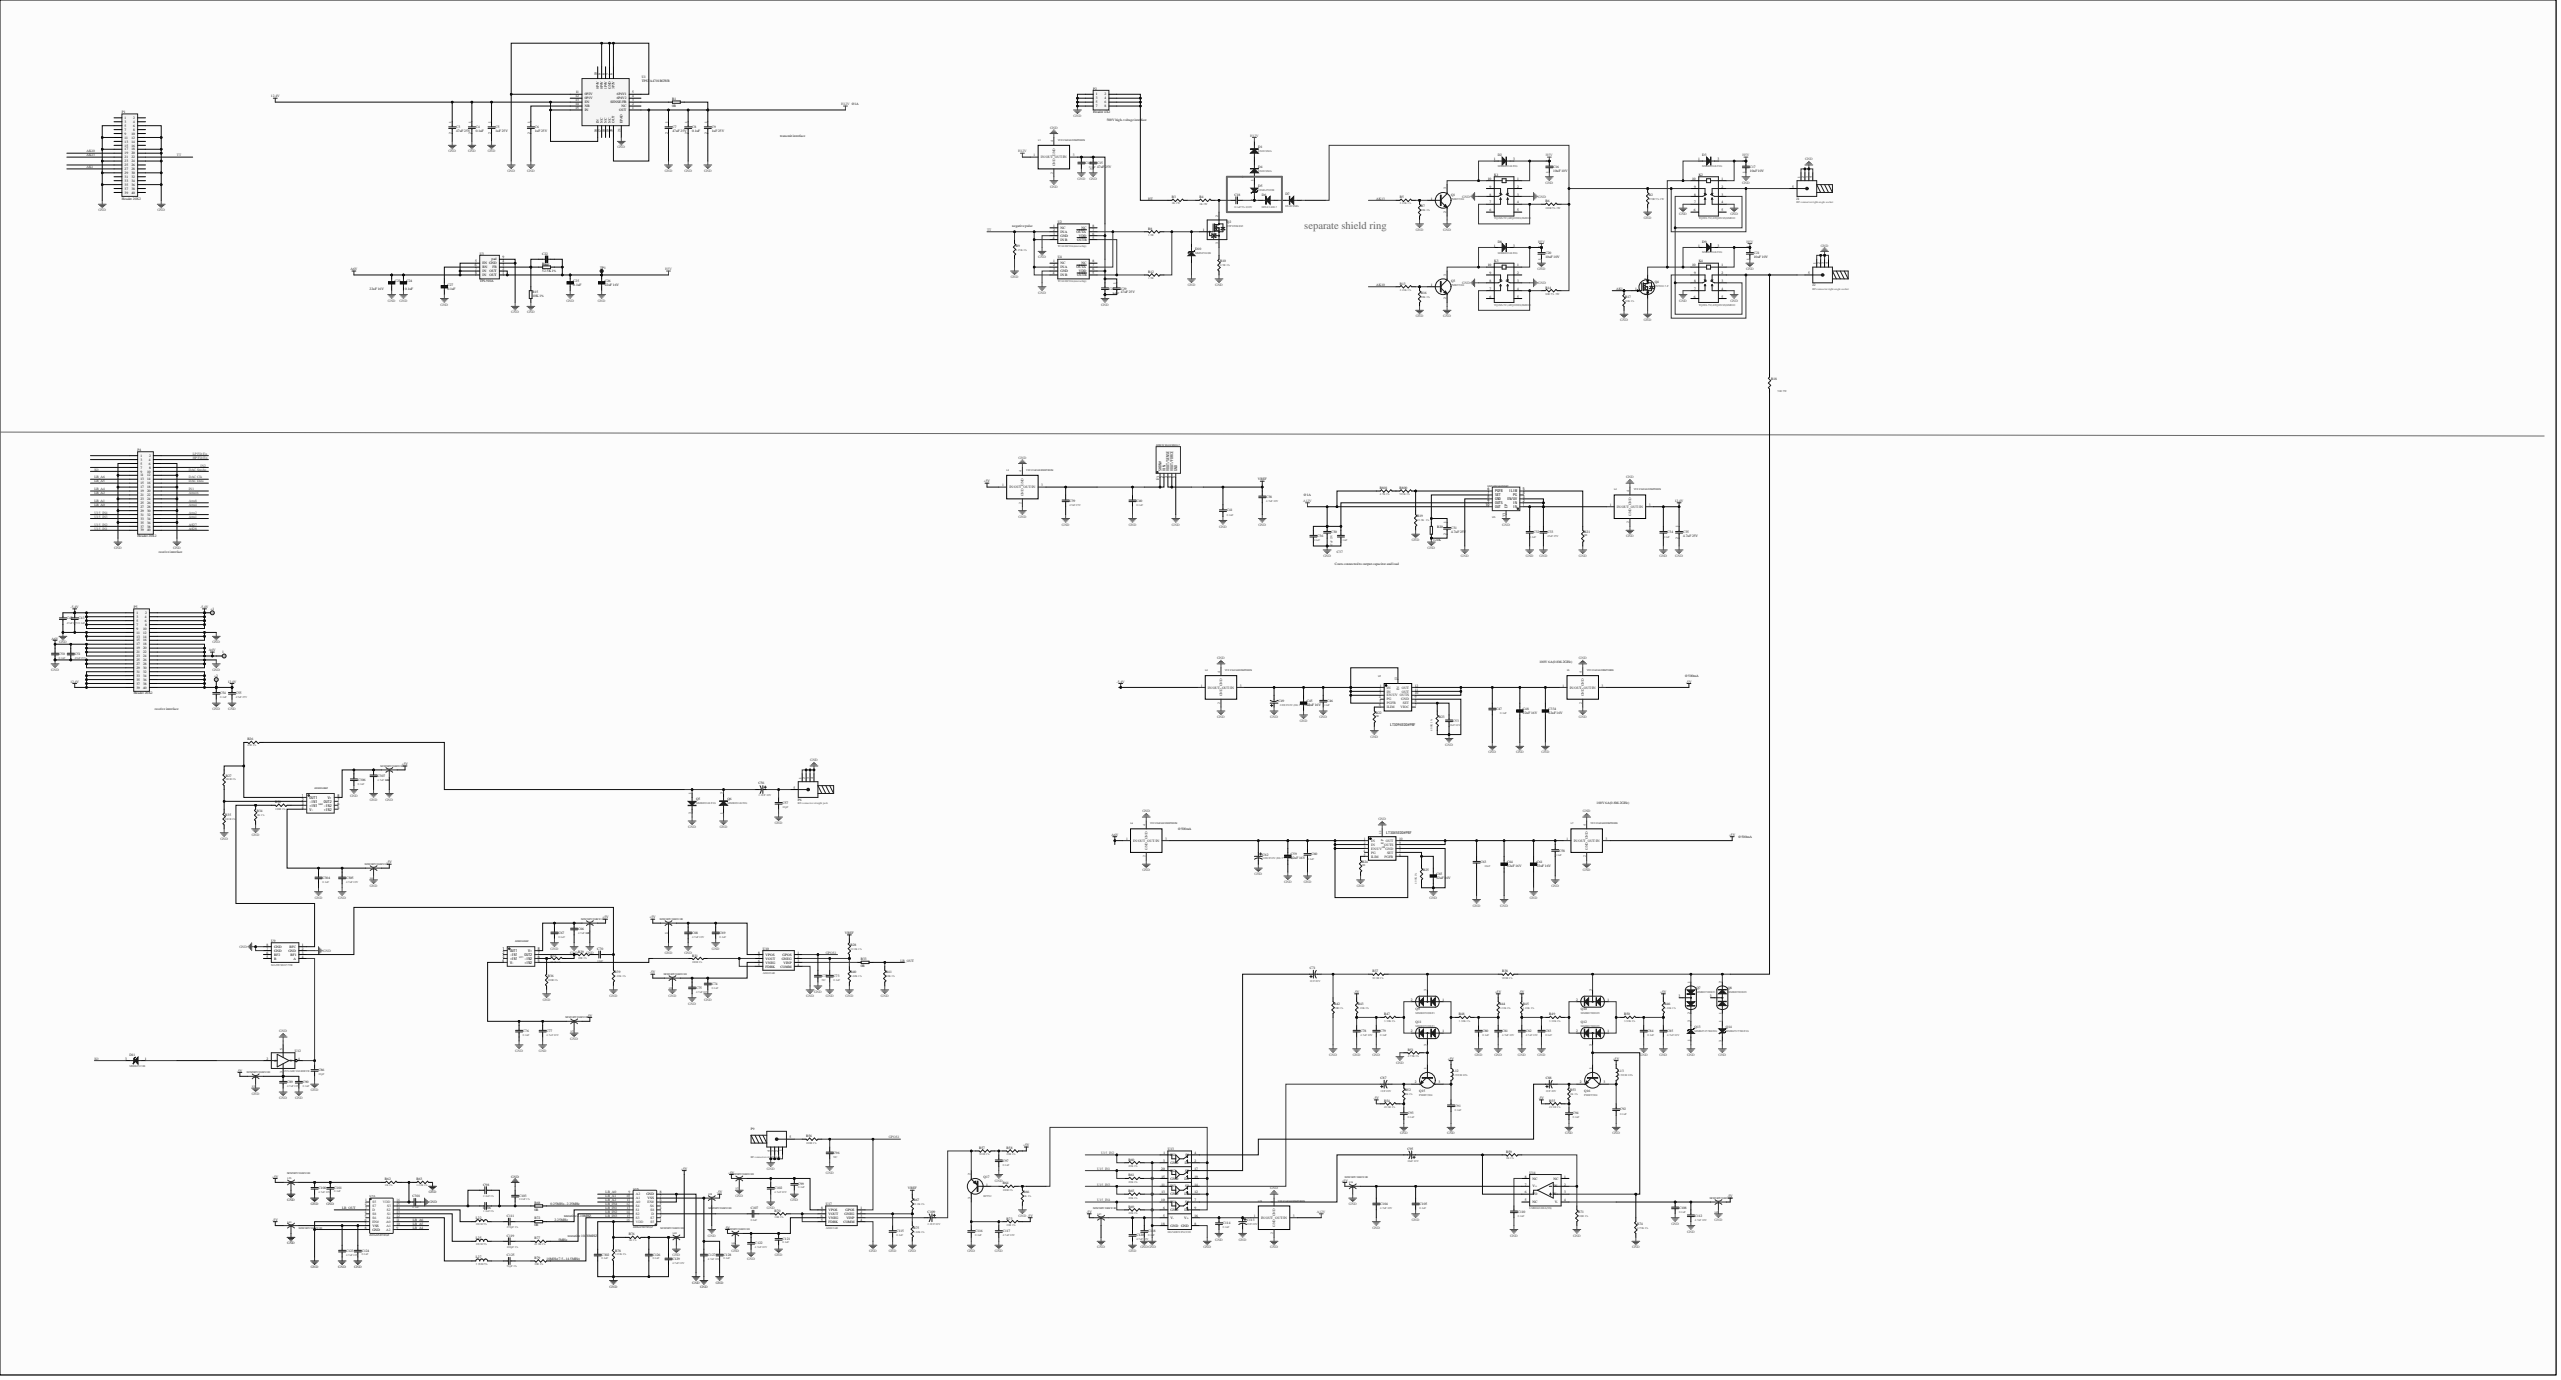Circuit board | Altium Designer | 299 parts | 156 nets
Bill of materials:
Comment,Description,Designator,Footprint,LibRef,Quantity
"","","+1, +2, 1","DIP-1","TP","3"
"47uF 25V","Capacitor","C3, C7, C15, C29, C30, C33, C39, C42, C51, C55","1206","CAP","10"
"0.1uF","Capacitor, [NoValue]","C4, C8, C14, C25, C28, C32, C34, C36, C37, C40, C41, C46, C47, C58, C60, C67, C69, C73, C74, C76, C79, C80, C83, C84, C90, C91, C92, C93, C94, C97, C99, C101, C105, C107, C108, C114, C115, C116, C118, C121, C124, C126, C128, C301, C302, C304, C306","0402","CAP, C1206","47"
"1uF 25V","Capacitor","C5, C6, C9","0402","CAP","3"
"10uF 10V","Capacitor","C16, C17, C20, C21","0603","CAP","4"
"0.1uF 5% 630V","Capacitor","C18","AXIAL0.59","CAP","1"
"10nF","[NoValue], Capacitor","C22, C70","0603","C1206, CAP","2"
"22uF 16V","[NoValue], Capacitor","C23, C26, C45, C48, C53, C59, C61, C64, C65, C334","0603","C1206, CAP","10"
"0.1uF","[NoValue], Capacitor","C24, C27, C43, C50, C54, C110","0603","C0402, CAP","6"
"4.7uF 25V","Capacitor","C31, C35","0603","CAP","2"
"4.7uF 10V","Capacitor","C38, C66, C68, C75, C77, C78, C81, C82, C85, C89, C100, C102, C104, C112, C117, C120, C122, C123, C127, C129, C305, C307","0402","CAP","22"
"220UF10V (D6.3*7.7mm)","Capacitor","C49, C62","CAP-SMD_BD6.3-L6.6-W6.6-FD","CAPACITOR_1","2"
"2.2UF 10V","Capacitor","C56, C109","0603钽电容","CAPACITOR","2"
"10pF","Capacitor","C57, C86","0402","CAP","2"
"10nF","Capacitor","C63","0402","CAP","1"
"1UF 20V","Capacitor","C71, C87, C88, C113","0603钽电容","CAPACITOR","4"
"NC","Capacitor","C72, C96","0603","CAP","2"
"10uF 10V","Capacitor","C95","0603钽电容","CAPACITOR","1"
"2.2nF 1%","Capacitor","C98, C103","0402","CAP","2"
"1.2nF 1%","Capacitor","C106","0402","CAP","1"
"270pF 1%","Capacitor","C111","0603","CAP","1"
"100pF 1%","Capacitor","C119","0603","CAP","1"
"56pF 1%","Capacitor","C125","0603","CAP","1"
"ES1D SMA","Diode","D1, D4, D7","1606D","DIODE","3"
"MMBD914LT1G","","D2, D3, D8, D9, Q5, Q6","SOT23","MMBD914LT1G","6"
"3SMAJ5929B","Zener Diode","D5","1606D","ZENER3","1"
"DFLU1400-7","Diode","D6","1606D","DIODE","1"
"MMSZ5248B","Zener Diode","D10","1206D","ZENER3","1"
"MMBZ5231B","","D11","SOT23","MMBZ5257BLT1G","1"
"RF connector right-angle socket","","J1, J2","DIP-P","JA1","2"
"TQ2SS-5V(ATQ209SS)SMD10","","K1, K2, K3, K4","K","TQ2SS-5V","4"
"YFF31HC2A105MT000N","","L1, L2, L3, L4, L5, L6, L7, L19","FILTER-SMD_4P-L3.2-W1.6-L_YFF31HC","YFF31HC2A105MT000N","8"
"NFM18PC104R1C3D","","L8, L9, L10, L11, L14, L15, L16, L17, L18, L20, L21, L23, L24, L26, L60, L61","FILTER-SMD_3P-L1.6-W0.8-L_NFM18CC223R1C3D","NFM15PC104R1A3D","16"
"0.39UH 10%","","L12, L13","0805","INDUCTOR","2"
"18UH 5%","","L22","0805","INDUCTOR","1"
"10UH 5%","","L25","0805","INDUCTOR","1"
"3.9UH 5%","","L27","0805","INDUCTOR","1"
"Header 20X2","Header, 20-Pin, Dual row","P1, P4, P5","N0.8mm/40Pin-Plug","Header 20X2","3"
"Header 4X2","Header, 4-Pin, Dual row","P2","N0.8mm/8Pin-SOCKET","Header 4X2","1"
"RF connector straight jack","","P6, P9","DIP-P","JA1","2"
"PMBT3904","NPN Transistor","Q1, Q3, Q15, Q16","SOT23","NPN","4"
"STP10NK80Z","","Q2","TO220","STP10NK80Z","1"
"2N7002-7-F","","Q4","SOT23","2N7002-7-F","1"
"MMBD7000LT1","Diode","Q7, Q8, Q9, Q10, Q11, Q12","SOT23","D1","6"
"MMBZ5257BLT1G","","Q13, Q14","SOT23","MMBZ5231B","2"
"BFT92","PNP Transistor","Q17","SOT23","PNP","1"
"0R","","R1, R21, R22, R24, R33, R68","0402","RES, RES1","6"
"470R 5% 1W","","R2","2512","RES1","1"
"1K 1W","","R3, R4","2512","RES1","2"
"2.21K 1%","","R5, R13","0603","RES1","2"
"220R 5% 1W","","R6","2512","RES1","1"
"10K 1%","","R7, R15, R16, R17, R41","0603","RES1, R0603","5"
"1.5R","","R8, R12","0603","RES1","2"
"1.15K 1%","","R9","1206","RES1","1"
"0.5R 1%","","R10","0805","RES1","1"
"52.5K 1%","","R11","0603","R0603","1"
"82R 5% 3W","","R14","2512","RES1","1"
"51R 5W","","R18","5W","RES1","1"
"13.3K  1%","","R19","0402","RES1","1"
"121K","","R20","0603","RES","1"
"49.9K 1%","","R23, R25","0402","RES1","2"
"47R 1%","","R26","0603","RES1","1"
"681R 1%","","R27, R32, R35","0603","RES1","3"
"22.1K 1%","","R28, R67","0603","RES1","2"
"10R 1%","","R29, R42, R70, R79","0603","RES1","4"
"100R 1%","","R30, R31, R36, R56, R64","0603","RES1","5"
"1K 1%","","R34, R52, R53, R59, R62, R66, R76","0603","RES1","7"
"90.9R 1%","","R37","1206","RES1","1"
"909R 1%","","R38","1206","RES1","1"
"1.21K 1%","","R39, R43, R44, R45, R46, R63, R78","0603","RES1","7"
"5.62K 1%","","R40, R75","0603","RES1","2"
"3.32K 1%","","R47, R48, R49, R50","0603","RES1","4"
"4.75K 1%","","R51, R74","0603","RES1","2"
"49.9R 1%","","R54, R55, R77","0603","RES1","3"
"301R 1%","","R57","0603","RES1","1"
"20R 1%","","R58, R73","0603","RES1","2"
"20K 1%","","R60, R61, R65, R69","0603","RES1","4"
"118R 1%","","R71","0603","RES1","1"
"0R","","R72","0603","RES","1"
"523K 1%","","R800","0402","RES1","1"
"4.7K 1%","","R801","0402","RES1","1"
"","","TP1","TP1","TEST_2","1"
"TPS7A4701RGWR","","U1","QFN-20","TPS7A4701RGWR(QFN20)","1"
"TC4426COA(microchip)","","U2, U4","SO8","TC4426COA","2"
"TPL910A","3PEAK","U3","DFN-8_L3.0-W3.0-P0.65-BL-EP2.3","TPL910A","1"
"GM12051ACPZ-R7","","U5","TDFN-10_L3.0-W3.0-P0.50-BL-EP","GM12051ACPZ-R7","1"
"ADR391AUJZ-REEL7","","U6","TSOT-23-5_L2.9-W1.6-P0.95-LS2.8-BR","ADR391AUJZ-REEL7","1"
"LT3094EDD#PBF","","U7","WDFN-12_L3.0-W3.0-P0.45-BL-EP","LT3094EDD#PBF","1"
"LT3045EDD#PBF","","U8","DFN-10_L3.0-W3.0-P0.50-BL-EP","LT3045EDD#PBF","1"
"MASWSS0157TR","","U9","SO8","MASWSS0157TR","1"
"AD603AR","","U10, U17","SO8","AD603AR","2"
"AD8002ARZ","","U11, U60","SOP8","AD8002ARZ","2"
"SN74AHC1G04DBVR","","U12","SOT25","SN74AHC1G04DBVR","1"
"DG540DN PLCC20","","U13","QUAD20","DG540DN","1"
"LMH6624MA(NS)","","U14","SO8","LMH6624MA","1"
"ADG658YRQZ","","U15, U16","TSSOP-16_L5.0-W4.4-P0.65-LS6.4-TL","ADG658YRQZ","2"
Netlist (Protel format):
[
1
DIP-1




]
[
+1
DIP-1




]
[
+2
DIP-1




]
[
C3
1206
47uF 25V



]
[
C4
0402
0.1uF



]
[
C5
0402
1uF 25V



]
[
C6
0402
1uF 25V



]
[
C7
1206
47uF 25V



]
[
C8
0402
0.1uF



]
[
C9
0402
1uF 25V



]
[
C14
0402
0.1uF



]
[
C15
1206
47uF 25V



]
[
C16
0603
10uF 10V



]
[
C17
0603
10uF 10V



]
[
C18
AXIAL0.59
0.1uF 5% 630V



]
[
C20
0603
10uF 10V



]
[
C21
0603
10uF 10V



]
[
C22
0603
10nF



]
[
C23
0603
22uF 16V



]
[
C24
0603
0.1uF



]
[
C25
0402
0.1uF



]
[
C26
0603
22uF 16V



]
[
C27
0603
0.1uF



]
[
C28
0402
0.1uF



]
[
C29
1206
47uF 25V



]
[
C30
1206
47uF 25V



]
[
C31
0603
4.7uF 25V



]
[
C32
0402
0.1uF



]
[
C33
1206
47uF 25V



]
[
C34
0402
0.1uF



]
[
C35
0603
4.7uF 25V



]
[
C36
0402
0.1uF



]
[
C37
0402
0.1uF



]
[
C38
0402
4.7uF 10V



]
[
C39
1206
47uF 25V



]
[
C40
0402
0.1uF



]
[
C41
0402
0.1uF



]
[
C42
1206
47uF 25V



]
[
C43
0603
0.1uF



]
[
C45
0603
22uF 16V



]
[
C46
0402
0.1uF



]
[
C47
0402
0.1uF



]
[
C48
0603
22uF 16V



]
[
C49
CAP-SMD_BD6.3-L6.6-W6.6-FD
220UF10V (D6.3*7.7mm)



]
[
C50
0603
0.1uF



]
[
C51
1206
47uF 25V



]
[
C53
0603
22uF 16V



]
[
C54
0603
0.1uF



]
[
C55
1206
47uF 25V



]
[
C56
0603钽电容
2.2UF 10V



]
[
C57
0402
10pF



]
[
C58
0402
0.1uF



]
[
C59
0603
22uF 16V



]
[
C60
0402
0.1uF



]
[
C61
0603
22uF 16V



]
[
C62
CAP-SMD_BD6.3-L6.6-W6.6-FD
220UF10V (D6.3*7.7mm)



]
[
C63
0402
10nF



]
[
C64
0603
22uF 16V



]
[
C65
0603
22uF 16V



]
[
C66
0402
4.7uF 10V



]
[
C67
0402
0.1uF



]
[
C68
0402
4.7uF 10V



]
[
C69
0402
0.1uF



]
[
C70
0603
10nF



]
[
C71
0603钽电容
1UF 20V



]
[
C72
0603
NC



]
[
C73
0402
0.1uF



]
[
C74
0402
0.1uF



]
[
C75
0402
4.7uF 10V



]
[
C76
0402
0.1uF



]
[
C77
0402
4.7uF 10V



]
[
C78
0402
4.7uF 10V



]
[
C79
0402
0.1uF



]
[
C80
0402
0.1uF



]
[
C81
0402
4.7uF 10V



]
[
C82
0402
4.7uF 10V



]
[
C83
0402
0.1uF



]
[
C84
0402
0.1uF



]
[
C85
0402
4.7uF 10V



]
[
C86
0402
10pF



]
[
C87
0603钽电容
1UF 20V



]
[
C88
0603钽电容
1UF 20V



]
[
C89
0402
4.7uF 10V



]
[
C90
0402
0.1uF



]
[
C91
0402
0.1uF



]
[
C92
0402
0.1uF



]
[
C93
0402
0.1uF



]
[
C94
0402
0.1uF



]
[
C95
0603钽电容
10uF 10V



]
[
C96
0603
NC



]
[
C97
0402
0.1uF



]
[
C98
0402
2.2nF 1%



]
[
C99
0402
0.1uF



]
[
C100
0402
4.7uF 10V



]
[
C101
0402
0.1uF



]
[
C102
0402
4.7uF 10V



]
[
C103
0402
2.2nF 1%



]
[
C104
0402
4.7uF 10V



]
[
C105
0402
0.1uF



]
[
C106
0402
1.2nF 1%



]
[
C107
0402
0.1uF



]
[
C108
0402
0.1uF



]
[
C109
0603钽电容
2.2UF 10V



]
[
C110
0603
0.1uF



]
[
C111
0603
270pF 1%



]
[
C112
0402
4.7uF 10V



]
[
C113
0603钽电容
1UF 20V



]
[
C114
0402
0.1uF



]
[
C115
0402
0.1uF



]
[
C116
0402
0.1uF



]
[
C117
0402
4.7uF 10V



]
[
C118
0402
0.1uF



]
[
C119
0603
100pF 1%



]
[
C120
0402
4.7uF 10V



]
[
C121
0402
0.1uF



]
[
C122
0402
4.7uF 10V



]
[
C123
0402
4.7uF 10V



]
[
C124
0402
0.1uF



]
[
C125
0603
56pF 1%



]
[
C126
0402
0.1uF



]
[
C127
0402
4.7uF 10V



]
[
C128
0402
0.1uF



]
[
C129
0402
4.7uF 10V



]
[
C301
0402
0.1uF



]
[
C302
0402
0.1uF



]
[
C304
0402
0.1uF



]
[
C305
0402
4.7uF 10V



]
[
C306
0402
0.1uF



]
[
C307
0402
4.7uF 10V



]
[
C334
0603
22uF 16V



]
[
D1
1606D
ES1D SMA



]
[
D2
SOT23
MMBD914LT1G



]
[
D3
SOT23
MMBD914LT1G



]
[
D4
1606D
ES1D SMA



]
[
D5
1606D
3SMAJ5929B



]
[
D6
1606D
DFLU1400-7



]
[
D7
1606D
ES1D SMA



]
[
D8
SOT23
MMBD914LT1G



]
[
D9
SOT23
MMBD914LT1G



]
[
D10
1206D
MMSZ5248B



]
[
D11
SOT23
MMBZ5231B



]
[
J1
DIP-P
RF connector right-angle socket



]
[
J2
DIP-P
RF connector right-angle socket



]
[
K1
K
TQ2SS-5V(ATQ209SS)SMD10



]
[
K2
K
TQ2SS-5V(ATQ209SS)SMD10



]
[
K3
K
TQ2SS-5V(ATQ209SS)SMD10



]
[
K4
K
TQ2SS-5V(ATQ209SS)SMD10



]
[
L1
FILTER-SMD_4P-L3.2-W1.6-L_YFF31HC
YFF31HC2A105MT000N



]
[
L2
FILTER-SMD_4P-L3.2-W1.6-L_YFF31HC
YFF31HC2A105MT000N



]
[
L3
FILTER-SMD_4P-L3.2-W1.6-L_YFF31HC
YFF31HC2A105MT000N



]
[
L4
FILTER-SMD_4P-L3.2-W1.6-L_YFF31HC
YFF31HC2A105MT000N



]
[
L5
FILTER-SMD_4P-L3.2-W1.6-L_YFF31HC
YFF31HC2A105MT000N



]
[
L6
FILTER-SMD_4P-L3.2-W1.6-L_YFF31HC
YFF31HC2A105MT000N



]
[
L7
FILTER-SMD_4P-L3.2-W1.6-L_YFF31HC
YFF31HC2A105MT000N



]
[
L8
FILTER-SMD_3P-L1.6-W0.8-L_NFM18CC223R1C3D
NFM18PC104R1C3D



]
[
L9
FILTER-SMD_3P-L1.6-W0.8-L_NFM18CC223R1C3D
NFM18PC104R1C3D



]
[
L10
FILTER-SMD_3P-L1.6-W0.8-L_NFM18CC223R1C3D
NFM18PC104R1C3D



]
[
L11
FILTER-SMD_3P-L1.6-W0.8-L_NFM18CC223R1C3D
NFM18PC104R1C3D



]
[
L12
0805
0.39UH 10%



]
[
L13
0805
0.39UH 10%



]
[
L14
FILTER-SMD_3P-L1.6-W0.8-L_NFM18CC223R1C3D
NFM18PC104R1C3D



]
[
L15
FILTER-SMD_3P-L1.6-W0.8-L_NFM18CC223R1C3D
NFM18PC104R1C3D



]
[
L16
FILTER-SMD_3P-L1.6-W0.8-L_NFM18CC223R1C3D
NFM18PC104R1C3D



]
[
L17
FILTER-SMD_3P-L1.6-W0.8-L_NFM18CC223R1C3D
NFM18PC104R1C3D



]
[
L18
FILTER-SMD_3P-L1.6-W0.8-L_NFM18CC223R1C3D
NFM18PC104R1C3D



]
[
L19
FILTER-SMD_4P-L3.2-W1.6-L_YFF31HC
YFF31HC2A105MT000N



]
[
L20
FILTER-SMD_3P-L1.6-W0.8-L_NFM18CC223R1C3D
NFM18PC104R1C3D



]
[
L21
FILTER-SMD_3P-L1.6-W0.8-L_NFM18CC223R1C3D
NFM18PC104R1C3D



]
[
L22
0805
18UH 5%



]
[
L23
FILTER-SMD_3P-L1.6-W0.8-L_NFM18CC223R1C3D
NFM18PC104R1C3D



]
[
L24
FILTER-SMD_3P-L1.6-W0.8-L_NFM18CC223R1C3D
NFM18PC104R1C3D



]
[
L25
0805
10UH 5%



]
[
L26
FILTER-SMD_3P-L1.6-W0.8-L_NFM18CC223R1C3D
NFM18PC104R1C3D



]
[
L27
0805
3.9UH 5%



]
[
L60
FILTER-SMD_3P-L1.6-W0.8-L_NFM18CC223R1C3D
NFM18PC104R1C3D



]
[
L61
FILTER-SMD_3P-L1.6-W0.8-L_NFM18CC223R1C3D
NFM18PC104R1C3D



]
[
P1
N0.8mm/40Pin-Plug
Header 20X2



]
[
P2
N0.8mm/8Pin-SOCKET
Header 4X2



]
[
P4
N0.8mm/40Pin-Plug
Header 20X2



]
[
P5
N0.8mm/40Pin-Plug
Header 20X2



]
[
P6
DIP-P
RF connector straight jack



]
[
P9
DIP-P
RF connector straight jack



]
[
Q1
SOT23
PMBT3904



]
[
Q2
TO220
STP10NK80Z



]
[
Q3
SOT23
PMBT3904



]
[
Q4
SOT23
2N7002-7-F



]
[
Q5
SOT23
MMBD914LT1G



]
[
Q6
SOT23
MMBD914LT1G



]
[
Q7
SOT23
MMBD7000LT1



]
[
Q8
SOT23
MMBD7000LT1



]
[
Q9
SOT23
MMBD7000LT1



]
[
Q10
SOT23
MMBD7000LT1



]
[
Q11
SOT23
MMBD7000LT1



]
[
Q12
SOT23
MMBD7000LT1



]
[
Q13
SOT23
MMBZ5257BLT1G



]
[
Q14
SOT23
MMBZ5257BLT1G



]
[
Q15
SOT23
PMBT3904



]
[
Q16
SOT23
PMBT3904



]
[
Q17
SOT23
BFT92



]
[
R1
0402
0R



]
[
R2
2512
470R 5% 1W



]
[
R3
2512
1K 1W



]
[
R4
2512
1K 1W



]
[
R5
0603
2.21K 1%



]
[
R6
2512
220R 5% 1W



]
[
R7
0603
10K 1%



]
[
R8
0603
1.5R



]
[
R9
1206
1.15K 1%



]
[
R10
0805
0.5R 1%



]
[
R11
0603
52.5K 1%



]
[
R12
0603
1.5R



]
[
R13
0603
2.21K 1%



]
[
R14
2512
82R 5% 3W



]
[
R15
0603
10K 1%



]
[
R16
0603
10K 1%



]
[
R17
0603
10K 1%



]
[
R18
5W
51R 5W



]
[
R19
0402
13.3K  1%



]
[
R20
0603
121K



]
[
R21
0402
0R



]
[
R22
0402
0R



]
[
R23
0402
49.9K 1%



]
[
R24
0402
0R



]
[
R25
0402
49.9K 1%



]
[
R26
0603
47R 1%



]
[
R27
0603
681R 1%



]
[
R28
0603
22.1K 1%



]
[
R29
0603
10R 1%



]
[
R30
0603
100R 1%



]
[
R31
0603
100R 1%



]
[
R32
0603
681R 1%



]
[
R33
0402
0R



]
[
R34
0603
1K 1%



]
[
R35
0603
681R 1%



]
[
R36
0603
100R 1%



]
[
R37
1206
90.9R 1%



]
[
R38
1206
909R 1%



]
[
R39
0603
1.21K 1%



]
[
R40
0603
5.62K 1%



]
[
R41
0603
10K 1%



]
[
R42
0603
10R 1%



]
[
R43
0603
1.21K 1%



]
[
R44
0603
1.21K 1%



]
[
R45
0603
1.21K 1%



]
[
R46
0603
1.21K 1%



]
[
R47
0603
3.32K 1%



]
[
R48
0603
3.32K 1%



]
[
R49
0603
3.32K 1%



]
[
R50
0603
3.32K 1%



]
[
R51
0603
4.75K 1%



]
[
R52
0603
1K 1%



]
[
R53
0603
1K 1%



]
[
R54
0603
49.9R 1%



]
[
R55
0603
49.9R 1%



]
[
R56
0603
100R 1%



]
[
R57
0603
301R 1%



]
[
R58
0603
20R 1%



]
[
R59
0603
1K 1%



]
[
R60
0603
20K 1%



]
[
R61
0603
20K 1%



]
[
R62
0603
1K 1%



]
[
R63
0603
1.21K 1%



]
[
R64
0603
100R 1%



]
[
R65
0603
20K 1%



]
[
R66
0603
1K 1%



]
[
R67
0603
22.1K 1%



]
[
R68
0402
0R



]
[
R69
0603
20K 1%



]
[
R70
0603
10R 1%



]
[
R71
0603
118R 1%



]
[
R72
0603
0R



]
[
R73
0603
20R 1%



]
[
R74
0603
4.75K 1%



]
[
R75
0603
5.62K 1%



]
[
R76
0603
1K 1%



]
[
R77
0603
49.9R 1%



]
[
R78
0603
1.21K 1%



]
[
R79
0603
10R 1%



]
[
R800
0402
523K 1%



]
[
R801
0402
4.7K 1%



]
[
TP1
TP1




]
[
U1
QFN-20
TPS7A4701RGWR



]
[
U2
SO8
TC4426COA(microchip)



]
[
U3
DFN-8_L3.0-W3.0-P0.65-BL-EP2.3
TPL910A



]
[
U4
SO8
TC4426COA(microchip)



]
[
U5
TDFN-10_L3.0-W3.0-P0.50-BL-EP
GM12051ACPZ-R7



]
[
U6
TSOT-23-5_L2.9-W1.6-P0.95-LS2.8-BR
ADR391AUJZ-REEL7



]
[
U7
WDFN-12_L3.0-W3.0-P0.45-BL-EP
LT3094EDD#PBF



]
[
U8
DFN-10_L3.0-W3.0-P0.50-BL-EP
LT3045EDD#PBF



]
[
U9
SO8
MASWSS0157TR



]
[
U10
SO8
AD603AR



]
[
U11
SOP8
AD8002ARZ



]
[
U12
SOT25
SN74AHC1G04DBVR



]
[
U13
QUAD20
DG540DN PLCC20



]
[
U14
SO8
LMH6624MA(NS)



]
[
U15
TSSOP-16_L5.0-W4.4-P0.65-LS6.4-TL
ADG658YRQZ



]
[
U16
TSSOP-16_L5.0-W4.4-P0.65-LS6.4-TL
ADG658YRQZ



]
[
U17
SO8
AD603AR



]
[
U60
SOP8
AD8002ARZ



]
(
VREF
C38-2
C41-2
R28-1
R67-2
U6-3
U6-4
)
(
U15_IN4
P4-31
R69-2
U13-10
)
(
U15_IN3
P4-33
R65-1
U13-11
)
(
U15_IN2
P4-37
R60-2
U13-1
)
(
U15_IN1
P4-39
R61-1
U13-20
)
(
TT
P1-22
R9-1
U2-2
U2-4
U4-2
U4-4
)
(
NetR800_1
R800-1
R801-2
)
(
NetR70_1
R70-1
U17-5
U17-7
)
(
NetR64_2
R64-2
R66-2
U13-2
U13-9
U13-12
U13-19
)
(
NetR59_1
R59-1
R71-2
U14-2
)
(
NetR33_2
R33-2
U10-3
)
(
NetR32_2
R32-2
R36-1
U11-6
)
(
NetR31_2
R31-2
U10-5
U10-7
)
(
NetR31_1
R31-1
U11-5
)
(
NetR30_2
R30-2
R34-1
U9-1
)
(
NetR30_1
R30-1
U60-3
)
(
NetR29_2
R29-2
R32-1
U11-7
)
(
NetR27_2
R27-2
R35-1
U60-2
)
(
NetR26_1
R26-1
R27-1
U60-1
)
(
NetR24_1
R24-1
U8-5
)
(
NetR22_1
R22-1
U7-6
)
(
NetR21_1
R21-1
U5-5
)
(
NetR19_1
R19-1
R800-2
U5-6
)
(
NetR12_2
R12-2
U2-5
U4-5
)
(
NetR8_2
R8-2
U2-7
U4-7
)
(
NetR3_1
R3-1
R4-1
)
(
NetR1_2
R1-2
U1-3
)
(
NetQ17_1
Q17-1
R64-1
)
(
NetQ12_3
Q12-3
Q16-1
R74-2
U14-3
)
(
NetQ11_3
Q11-3
Q15-1
R51-1
)
(
NetQ10_2
Q10-2
Q12-2
R49-2
)
(
NetQ10_1
Q10-1
Q12-1
R50-1
)
(
NetQ9_3
Q9-3
R37-2
R38-1
)
(
NetQ9_2
Q9-2
Q11-2
R47-1
)
(
NetQ9_1
Q9-1
Q11-1
R48-2
)
(
NetQ8_1
Q8-1
Q14-1
)
(
NetQ7_2
Q7-2
Q13-3
)
(
NetQ7_1
Q7-1
Q8-2
Q10-3
R18-2
R38-2
)
(
NetQ3_1
Q3-1
R13-1
R16-1
)
(
NetQ2_3
Q2-3
R10-2
)
(
NetQ1_1
Q1-1
R5-1
R7-1
)
(
NetP9_5
P9-5
R56-2
)
(
NetL27_2
L27-2
U16-12
)
(
NetL25_2
L25-2
U16-13
)
(
NetL22_2
L22-2
U16-14
)
(
NetK3_4
K3-4
K3-7
R14-1
)
(
NetK2_3
K2-3
K2-8
K4-3
K4-8
)
(
NetK1_4
K1-4
K1-7
R6-1
)
(
NetJ2_5
J2-5
K4-2
K4-9
R18-1
)
(
NetD11_1
D11-1
U12-2
)
(
NetD10_2
D10-2
Q2-1
R8-1
R12-1
)
(
NetD8_1
D8-1
K3-10
Q3-3
)
(
NetD7_1
D7-1
J1-5
K2-2
K2-9
R2-1
R6-2
R14-2
)
(
NetD6_1
D6-1
D7-2
)
(
NetD4_1
D4-1
D5-1
)
(
NetD3_1
D3-1
D9-1
K2-10
K4-10
Q4-3
)
(
NetD2_1
D2-1
K1-10
Q1-3
)
(
NetD1_1
D1-1
D4-2
)
(
NetC306_1
C306-1
C307-2
L60-1
U60-8
)
(
NetC304_1
C304-1
C305-2
L61-1
U60-4
)
(
NetC302_2
C302-2
R76-1
R78-1
U15-16
)
(
NetC301_1
C301-1
R62-1
R63-2
U16-16
)
(
NetC127_2
C127-2
C128-2
L18-1
U15-7
)
(
NetC126_2
C126-2
C129-2
L24-1
R76-2
)
(
NetC125_2
C125-2
R79-1
)
(
NetC125_1
C125-1
L27-1
)
(
NetC123_2
C123-2
C124-1
L23-3
U16-7
)
(
NetC121_2
C121-2
C122-2
L26-3
U17-6
)
(
NetC119_2
C119-2
R77-1
)
(
NetC119_1
C119-1
L25-1
)
(
NetC118_2
C118-2
C120-2
L21-3
U13-5
)
(
NetC116_2
C116-2
C117-2
Q17-3
R73-1
)
(
NetC115_1
C115-1
R67-1
R75-2
U17-2
)
(
NetC113_1
C113-1
C114-2
L19-1
U13-16
)
(
NetC111_2
C111-2
R72-2
)
(
NetC111_1
C111-1
L22-1
)
(
NetC110_2
C110-2
U14-8
)
(
NetC109_2
C109-2
U17-3
)
(
NetC109_1
C109-1
Q17-2
R57-1
)
(
NetC108_2
C108-2
C112-2
L20-1
U14-4
)
(
NetC107_2
C107-2
R70-2
)
(
NetC107_1
C107-1
U15-3
)
(
NetC104_2
C104-2
C105-2
L16-3
U14-7
)
(
NetC100_2
C100-2
C101-1
L15-3
R62-2
)
(
NetC99_2
C99-2
C102-2
L17-3
U17-8
)
(
NetC98_2
C98-2
C103-2
C106-2
R68-2
)
(
NetC98_1
C98-1
C106-1
U16-15
)
(
NetC97_2
C97-2
R57-2
R58-2
)
(
NetC95_2
C95-2
U13-7
)
(
NetC95_1
C95-1
R59-2
U14-6
)
(
NetC94_2
C94-2
R53-1
R55-2
)
(
NetC93_2
C93-2
R52-2
R54-1
)
(
NetC92_1
C92-1
L13-2
Q16-3
)
(
NetC91_1
C91-1
L12-2
Q15-3
)
(
NetC89_2
C89-2
C90-1
L14-3
U12-3
)
(
NetC88_2
C88-2
Q16-2
R53-2
)
(
NetC88_1
C88-1
U13-4
)
(
NetC87_2
C87-2
Q15-2
R52-1
)
(
NetC87_1
C87-1
U13-14
)
(
NetC86_1
C86-1
U9-4
U12-4
)
(
NetC84_2
C84-2
C85-2
R46-2
R50-2
)
(
NetC82_2
C82-2
C83-1
R45-2
R49-1
)
(
NetC80_1
C80-1
C81-2
R44-2
R48-1
)
(
NetC78_2
C78-2
C79-2
R43-1
R47-2
)
(
NetC76_1
C76-1
C77-2
L11-1
U11-4
)
(
NetC74_1
C74-1
C75-2
L10-3
U10-6
)
(
NetC73_1
C73-1
R28-2
R40-2
U10-2
)
(
NetC71_2
C71-2
R37-1
R42-2
)
(
NetC71_1
C71-1
U13-17
)
(
NetC70_2
C70-2
R29-1
)
(
NetC70_1
C70-1
R39-1
U9-3
)
(
NetC68_2
C68-2
C69-1
L9-3
U10-8
)
(
NetC66_2
C66-2
C67-1
L8-1
U11-8
)
(
NetC65_2
C65-2
R25-1
U8-7
)
(
NetC59_2
C59-2
C60-1
C62-1
L6-3
U8-1
U8-2
U8-3
U8-6
)
(
NetC58_1
C58-1
C61-2
C63-1
C64-2
L7-1
U8-9
U8-10
)
(
NetC56_2
C56-2
Q5-1
Q6-3
R26-2
)
(
NetC56_1
C56-1
C57-2
P6-5
)
(
NetC53_1
C53-1
R23-1
U7-8
)
(
NetC47_1
C47-1
C48-2
C334-2
L5-1
U7-10
U7-11
U7-12
)
(
NetC45_2
C45-2
C46-1
C49-2
L4-3
U7-1
U7-2
U7-3
U7-5
U7-13
)
(
NetC39_1
C39-1
C40-2
L3-3
U6-1
U6-2
)
(
NetC32_1
C32-1
C33-1
L2-1
U5-1
U5-2
U5-3
)
(
NetC31_1
C31-1
R20-1
U5-7
)
(
NetC27_1
C27-1
U3-6
)
(
NetC22_1
C22-1
R11-1
R15-1
U3-3
)
(
NetC18_2
C18-2
D5-2
D6-2
)
(
NetC18_1
C18-1
Q2-2
R4-2
)
(
NetC14_1
C14-1
C15-1
C28-1
C29-1
L1-3
U2-6
U4-6
)
(
NetC6_1
C6-1
U1-14
)
(
LB_OUT
R33-1
R41-2
U16-3
)
(
LB_IN4
R68-1
U15-12
)
(
LB_IN3
R79-2
U15-15
)
(
LB_IN2
R77-2
U15-14
)
(
LB_IN1
R72-1
U15-13
)
(
LB_A6
P4-13
U16-11
)
(
LB_A5
P4-15
U16-10
)
(
LB_A4
P4-19
U16-9
)
(
LB_A2
P4-21
U15-11
)
(
LB_A1
P4-25
U15-10
)
(
LB_A0
P4-27
U15-9
)
(
K0
D11-3
P4-9
)
(
HT
P2-2
P2-4
P2-6
P2-8
R3-2
)
(
H12V
C7-1
C8-1
C9-1
D1-2
L1-1
R1-1
U1-1
U1-20
)
(
H5V
C16-2
C17-2
C20-2
C21-2
C22-2
C25-1
C26-1
D2-3
D3-3
D8-3
D9-3
K1-1
K2-1
K3-1
K4-1
R11-2
TP1-1
U3-1
U3-2
)
(
GPOS1
C72-1
C96-1
R56-1
U10-1
U17-1
)
(
GND
C3-2
C4-2
C5-2
C6-2
C7-2
C8-2
C9-2
C14-2
C15-2
C16-1
C17-1
C20-1
C21-1
C23-1
C24-2
C25-2
C26-2
C27-2
C28-2
C29-2
C30-2
C31-2
C32-2
C33-2
C34-2
C35-2
C36-2
C37-2
C38-1
C39-2
C40-1
C41-1
C42-2
C43-2
C45-1
C46-2
C47-2
C48-1
C49-1
C50-1
C51-2
C53-2
C54-2
C55-2
C57-1
C58-2
C59-1
C60-2
C61-1
C62-2
C63-2
C64-1
C65-1
C66-1
C67-2
C68-1
C69-2
C72-2
C73-2
C74-2
C75-1
C76-2
C77-1
C78-1
C79-1
C80-2
C81-1
C82-1
C83-2
C84-1
C85-1
C86-2
C89-1
C90-2
C91-2
C92-2
C93-1
C94-1
C96-2
C97-1
C99-1
C100-1
C101-2
C102-1
C103-1
C104-1
C105-1
C108-1
C110-1
C112-1
C113-2
C114-1
C115-2
C116-1
C117-1
C118-1
C120-1
C121-1
C122-1
C123-1
C124-2
C126-1
C127-1
C128-1
C129-1
C301-2
C302-1
C304-2
C305-1
C306-2
C307-1
C334-1
D10-1
J1-1
J1-2
J1-3
J1-4
J2-1
J2-2
J2-3
J2-4
K1-3
K1-8
K2-4
K2-7
K3-3
K3-8
K4-4
K4-7
L1-2
L1-4
L2-2
L2-4
L3-2
L3-4
L4-2
L4-4
L5-2
L5-4
L6-2
L6-4
L7-2
L7-4
L8-2
L9-2
L10-2
L11-2
L14-2
L15-2
L16-2
L17-2
L18-2
L19-2
L19-4
L20-2
L21-2
L23-2
L24-2
L26-2
L60-2
L61-2
P1-5
P1-6
P1-11
P1-12
P1-17
P1-18
P1-20
P1-23
P1-24
P1-29
P1-30
P1-35
P1-36
P2-1
P2-3
P2-5
P2-7
P4-5
P4-6
P4-11
P4-12
P4-17
P4-18
P4-23
P4-24
P4-29
P4-30
P4-35
P4-36
P5-11
P5-12
P5-13
P5-14
P5-15
P5-16
P5-25
P5-26
P5-27
P5-28
P5-29
P5-30
P6-1
P6-2
P6-3
P6-4
P9-1
P9-2
P9-3
P9-4
Q1-2
Q3-2
Q4-2
Q5-3
Q6-1
Q13-1
Q14-3
R2-2
R7-2
R9-2
R10-1
R15-2
R16-2
R17-1
R19-2
R20-2
R21-2
R22-2
R23-2
R24-2
R25-2
R34-2
R35-2
R36-2
R39-2
R40-1
R41-1
R42-1
R51-2
R60-1
R61-2
R63-1
R65-2
R66-1
R69-1
R71-1
R74-1
R75-1
R78-2
U1-5
U1-6
U1-7
U1-9
U1-11
U1-21
U2-3
U3-4
U3-9
U4-3
U5-8
U5-11
U6-5
U7-9
U8-8
U8-11
U9-2
U9-7
U9-8
U10-4
U12-5
U13-3
U13-6
U13-8
U13-13
U13-15
U13-18
U15-6
U15-8
U16-6
U16-8
U17-4
)
(
AK13
P1-21
R5-2
)
(
AK10
P1-19
R13-2
)
(
AK1
P1-27
Q4-1
R17-2
)
(
A12V
C30-1
C36-1
C37-1
L19-3
R801-1
U5-9
U5-10
)
(
A6V
1-1
C23-2
C24-1
C50-2
C51-1
L6-1
P5-17
P5-18
P5-19
P5-20
P5-21
P5-22
P5-23
P5-24
U3-5
U3-7
U3-8
)
(
-5V
L5-3
L10-1
L11-3
L14-1
L18-3
L20-3
L21-1
L23-1
L26-1
L61-3
R43-2
R45-1
R54-2
R55-1
R73-2
)
(
-5.4V
+1-1
C42-1
C43-1
L4-1
P5-1
P5-2
P5-3
P5-4
P5-5
P5-6
P5-7
P5-8
P5-9
P5-10
)
(
+5V
L3-1
L7-3
L8-3
L9-1
L12-1
L13-1
L15-1
L16-1
L17-1
L24-3
L60-3
R44-1
R46-1
R58-1
)
(
12.4V
+2-1
C3-1
C4-1
C5-1
C34-1
C35-1
C54-1
C55-1
L2-3
P5-31
P5-32
P5-33
P5-34
P5-35
P5-36
P5-37
P5-38
P5-39
P5-40
U1-13
U1-15
U1-16
)